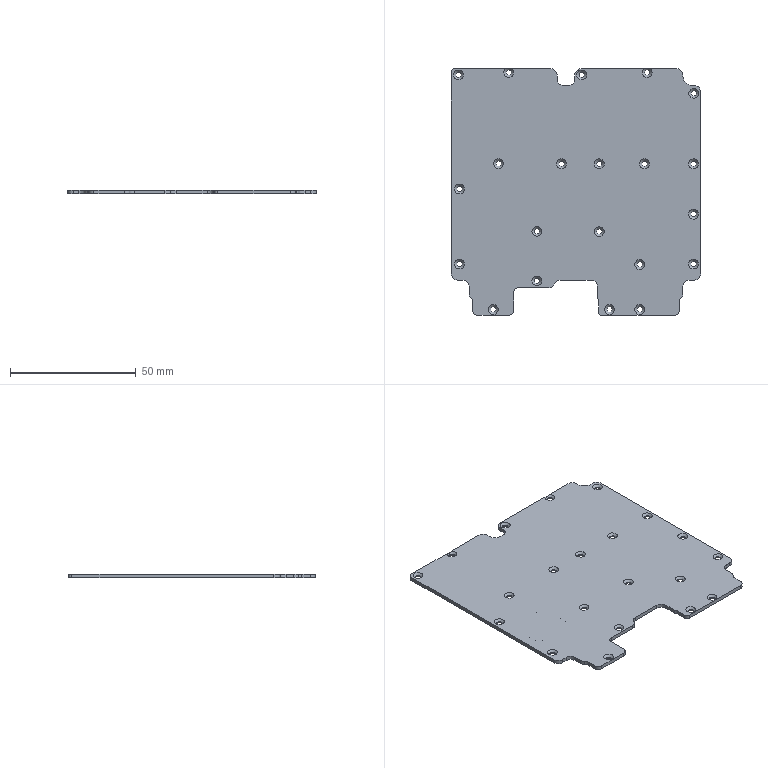Part | STEP file | Driver amplifier module cover | 1 solid | 121 faces | box 99 x 98 x 1.5 mm | volume 12973 mm3 | cylinder 50 | cone 42 | plane 29 | commonest cylinder face diameters 2.2 x21 5 x15 4 x11 2.54 x2 7.359 x1